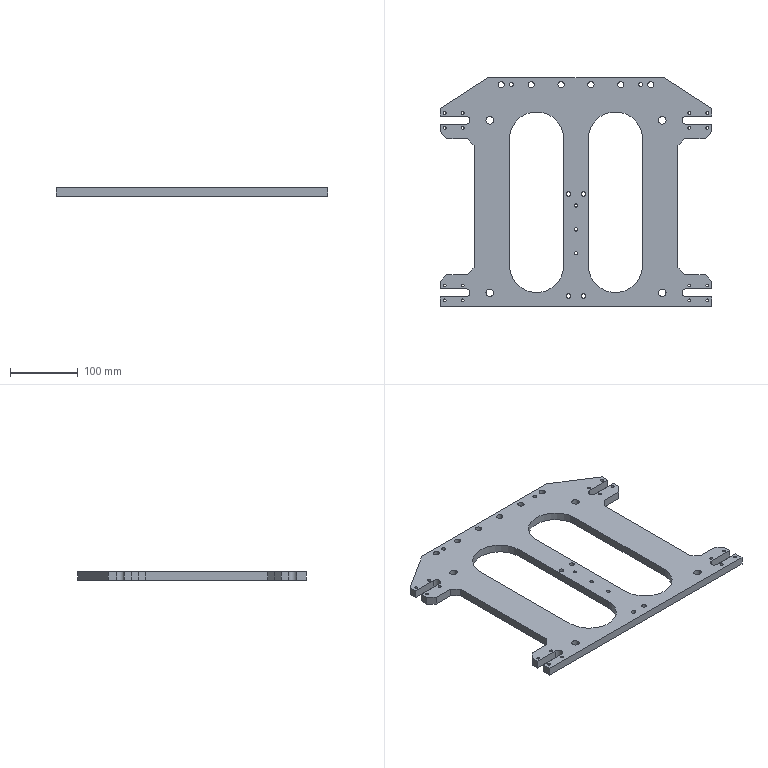NC program | NX | posted with a generic post | part box 400 x 336 x 12 mm
Lines 4690 to 4851 of 4851:
(ZLEVEL_PROFILE_COPY_COPY_1_1 , TOOL : D10JING)
N9378 T09 M6
N9380 G54
N9382 G17 G0 G90 X209.485 Y126.167 S5000 M3
N9384 G43 Z80. H9
N9386 Z-9.
N9388 G94 G1 Z-12. F1200.
N9390 X205.5 Y123.866
N9392 G3 X205. Y123. R1.
N9394 G1 Y111.5
N9396 G2 X200. Y106.5 R5.
N9398 G1 X162.
N9400 G3 X161. Y105.5 R1.
N9402 X162. Y104.5 R1.
N9404 G1 X200.
N9406 G2 X205. Y99.5 R5.
N9408 G1 Y88.5
N9410 G2 X203.536 Y84.964 R5.
N9412 G1 X193.536 Y74.964
N9414 G2 X190. Y73.5 R5.
N9416 G1 X162.071
N9418 X155. Y66.429
N9420 Y-109.429
N9422 X162.071 Y-116.5
N9424 X190.
N9426 G2 X193.536 Y-117.964 R5.
N9428 G1 X203.536 Y-127.964
N9430 G2 X205. Y-131.5 R5.
N9432 G1 Y-142.5
N9434 G2 X200. Y-147.5 R5.
N9436 G1 X162.
N9438 G3 X161. Y-148.5 R1.
N9440 X162. Y-149.5 R1.
N9442 G1 X200.
N9444 G2 X205. Y-154.5 R5.
N9446 G1 Y-168.
N9448 G3 X205.5 Y-168.866 R1.
N9450 G1 X209.485 Y-171.167
N9452 Z-9.
N9454 G0 Z80.
N9456 X-209.485
N9458 Z-9.
N9460 G1 Z-12.
N9462 X-205.5 Y-168.866
N9464 G3 X-205. Y-168. R1.
N9466 G1 Y-154.5
N9468 G2 X-200. Y-149.5 R5.
N9470 G1 X-162.
N9472 G3 X-161. Y-148.5 R1.
N9474 X-162. Y-147.5 R1.
N9476 G1 X-200.
N9478 G2 X-205. Y-142.5 R5.
N9480 G1 Y-131.5
N9482 G2 X-203.536 Y-127.964 R5.
N9484 G1 X-193.536 Y-117.964
N9486 G2 X-190. Y-116.5 R5.
N9488 G1 X-162.071
N9490 X-155. Y-109.429
N9492 Y66.429
N9494 X-162.071 Y73.5
N9496 X-190.
N9498 G2 X-193.536 Y74.964 R5.
N9500 G1 X-203.536 Y84.964
N9502 G2 X-205. Y88.5 R5.
N9504 G1 Y99.5
N9506 G2 X-200. Y104.5 R5.
N9508 G1 X-162.
N9510 G3 X-161. Y105.5 R1.
N9512 X-162. Y106.5 R1.
N9514 G1 X-200.
N9516 G2 X-205. Y111.5 R5.
N9518 G1 Y123.
N9520 G3 X-205.5 Y123.866 R1.
N9522 G1 X-209.485 Y126.167
N9524 Z-9.
N9526 G0 Z80.
N9528 M5
(ZLEVEL_PROFILE_COPY_COPY_COPY , TOOL : D6A45)
N9530 T07 M6
N9532 G54
N9534 G17 G0 G90 X-201.904 Y-170.421 S7500 M3
N9536 G43 Z80. H7
N9538 Z2.
N9540 G94 G1 Z-1. F1200.
N9542 X-201.212 Y-170.019
N9544 G3 X-200.913 Y-169.499 R0.6
N9546 G1 X-200.917 Y-167.987
N9548 Y-154.499
N9550 G2 X-200.001 Y-153.583 R0.916
N9552 G1 X-162.
N9554 G3 X-156.917 Y-148.5 R5.083
N9556 X-162. Y-143.417 R5.083
N9558 G1 X-200.001
N9560 G2 X-200.917 Y-142.501 R0.925
N9562 G1 Y-131.499
N9564 G2 X-200.649 Y-130.852 R0.915
N9566 G1 X-190.648 Y-120.851
N9568 G2 X-190.001 Y-120.583 R0.916
N9570 G1 X-160.38
N9572 X-150.917 Y-111.12
N9574 Y68.12
N9576 X-160.38 Y77.583
N9578 X-190.003
N9580 G2 X-190.648 Y77.851 R0.912
N9582 G1 X-200.649 Y87.852
N9584 G2 X-200.917 Y88.499 R0.952
N9586 G1 Y99.501
N9588 G2 X-200.001 Y100.417 R0.916
N9590 G1 X-162.
N9592 G3 X-156.917 Y105.5 R5.083
N9594 X-162. Y110.583 R5.083
N9596 G1 X-200.001
N9598 G2 X-200.917 Y111.499 R0.928
N9600 G1 Y124.617
N9602 G3 X-201.217 Y125.136 R0.6
N9604 G1 X-201.963 Y125.567
N9606 Z2.
N9608 G0 Z80.
N9610 X201.85 Y125.81
N9612 Z2.
N9614 G1 Z-1.
N9616 X201.154 Y125.325
N9618 G3 X200.899 Y124.781 R0.6
N9620 G1 X200.917 Y124.566
N9622 Y111.499
N9624 G2 X200.001 Y110.583 R0.928
N9626 G1 X162.
N9628 G3 X156.917 Y105.5 R5.083
N9630 X162. Y100.417 R5.083
N9632 G1 X200.001
N9634 G2 X200.917 Y99.501 R0.916
N9636 G1 Y88.499
N9638 G2 X200.649 Y87.852 R0.952
N9640 G1 X190.648 Y77.851
N9642 G2 X190.003 Y77.583 R0.912
N9644 G1 X160.38
N9646 X150.917 Y68.12
N9648 Y-111.12
N9650 X160.38 Y-120.583
N9652 X190.001
N9654 G2 X190.648 Y-120.851 R0.916
N9656 G1 X200.649 Y-130.852
N9658 G2 X200.917 Y-131.499 R0.915
N9660 G1 Y-142.501
N9662 G2 X200.001 Y-143.417 R0.925
N9664 G1 X162.
N9666 G3 X156.917 Y-148.5 R5.083
N9668 X162. Y-153.583 R5.083
N9670 G1 X200.001
N9672 G2 X200.917 Y-154.499 R0.916
N9674 G1 Y-167.987
N9676 Y-169.483
N9678 G3 X201.217 Y-170.002 R0.6
N9680 G1 X201.914 Y-170.405
N9682 Z2.
N9684 G0 Z80.
N9686 M5
N9688 M2